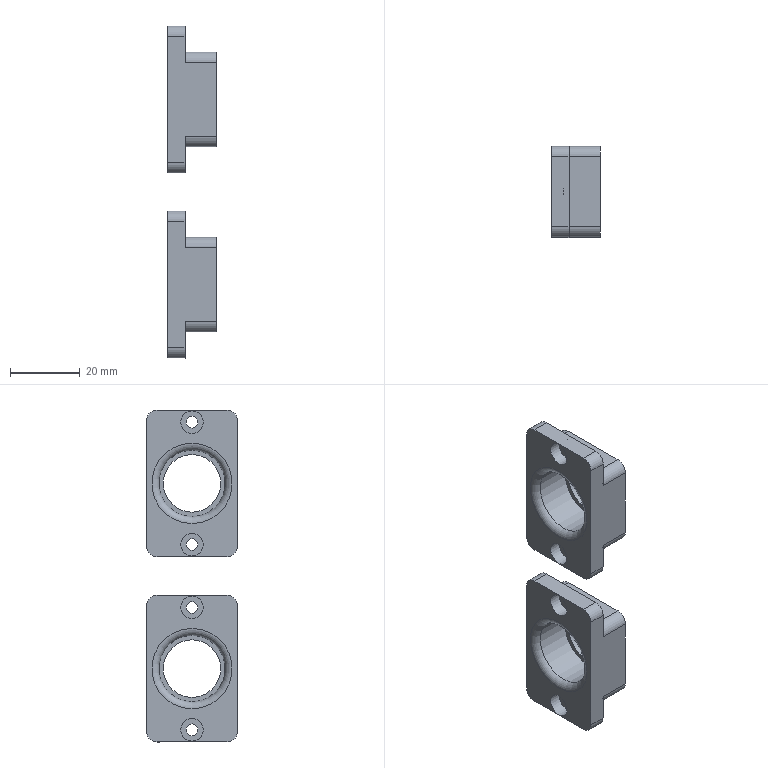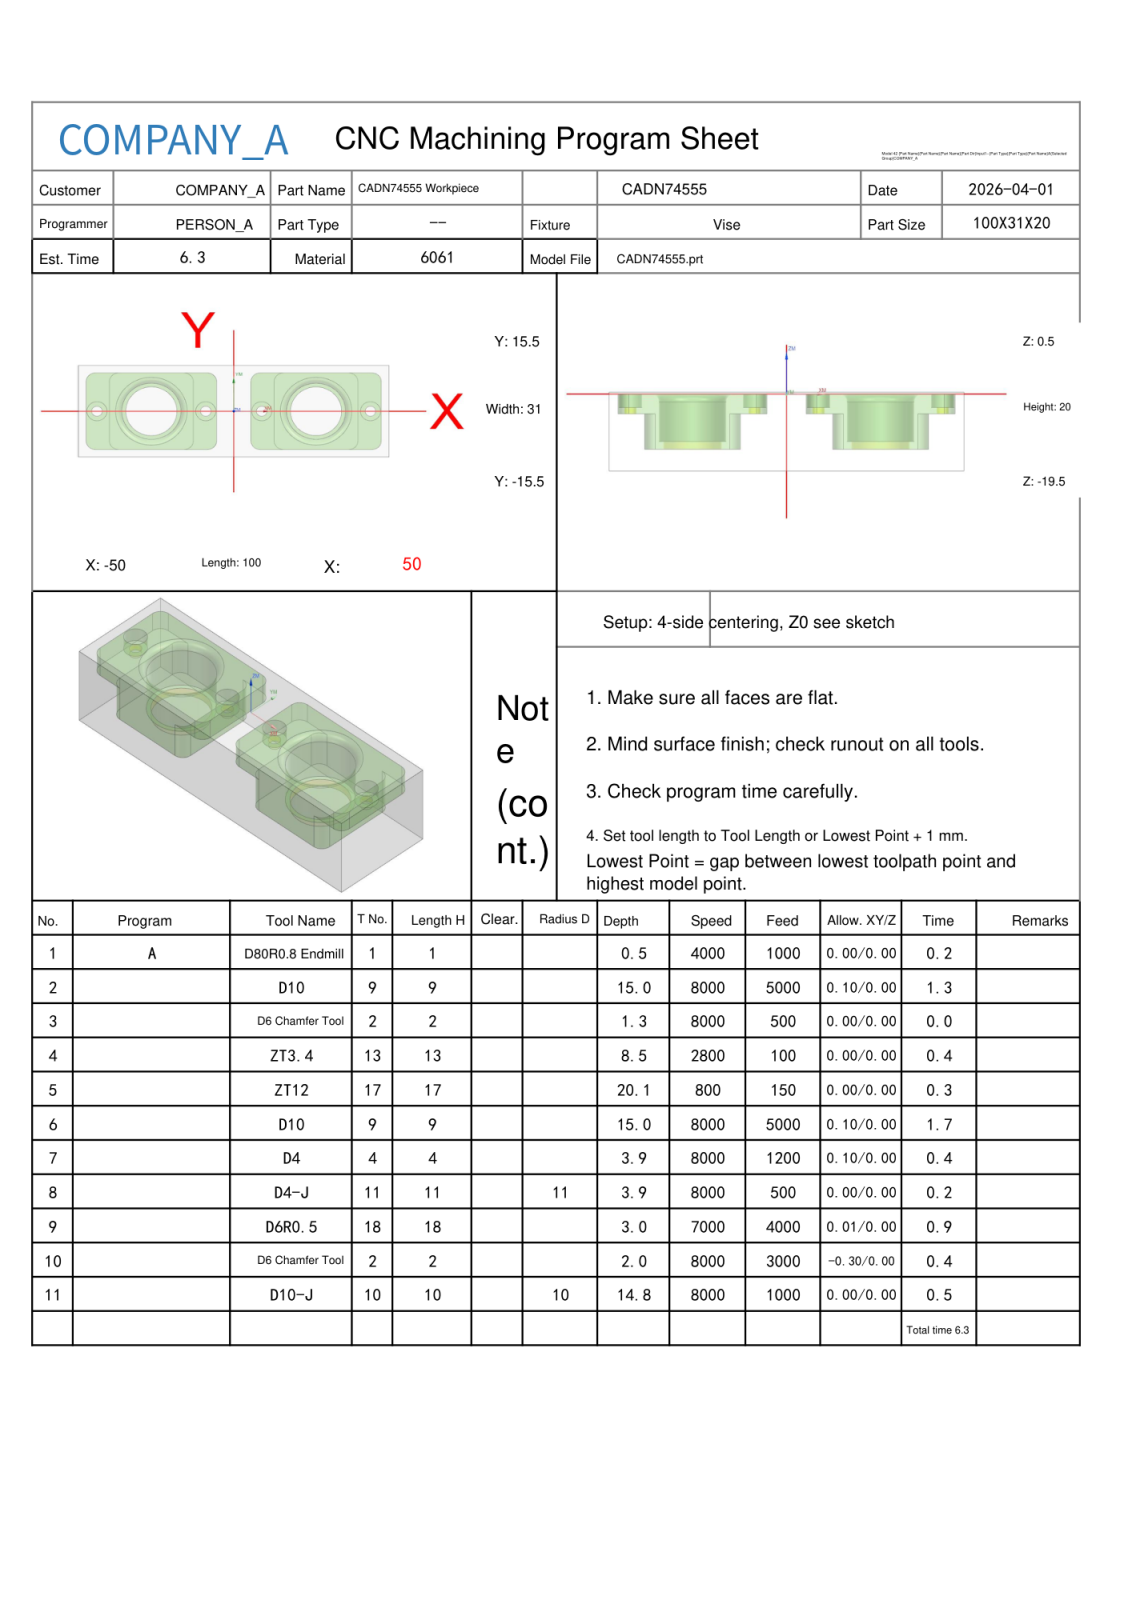NC program | NX | posted by the shop | part box 14 x 26 x 95 mm
Lines 5543 to 6944 of 19918:
N9 T18 M06
(D6R0.5  D=6. R=0.5 H=18 ce=0.01 di=0.00)
G00 G90 G54 X-25.418 Y8.734 M03 S7000
G43 H18 Z20.
M08
Z1.5
G01 X-25.945 Y8.792 Z1.472 F4000.
X-26.768 Y8.806 Z1.429
X-27.589 Y8.742 Z1.386
X-28.401 Y8.602 Z1.343
X-29.195 Y8.387 Z1.3
X-29.967 Y8.099 Z1.256
X-30.708 Y7.74 Z1.213
X-31.412 Y7.313 Z1.17
X-32.073 Y6.823 Z1.127
X-32.686 Y6.273 Z1.084
X-33.245 Y5.668 Z1.041
X-33.744 Y5.013 Z.998
X-34.066 Y4.514 Z.966
X-34.46 Y3.775 Z.923
X-34.782 Y3.003 Z.879
X-35.03 Y2.203 Z.835
X-35.201 Y1.384 Z.791
X-35.293 Y.552 Z.747
X-35.305 Y-.285 Z.703
X-35.238 Y-1.12 Z.659
X-35.093 Y-1.944 Z.615
X-34.869 Y-2.751 Z.572
X-34.57 Y-3.533 Z.528
X-34.199 Y-4.283 Z.484
X-33.757 Y-4.994 Z.44
X-33.251 Y-5.661 Z.396
X-32.683 Y-6.276 Z.352
X-32.059 Y-6.834 Z.308
X-31.385 Y-7.331 Z.264
X-30.668 Y-7.762 Z.221
X-29.912 Y-8.122 Z.177
X-29.126 Y-8.41 Z.133
X-28.316 Y-8.621 Z.089
X-27.731 Y-8.723 Z.058
X-27.265 Y-8.777 Z.033
X-26.797 Y-8.805 Z.009
X-26.5 Z-.007
G03 X-17.695 Y0.0 I0.0 J8.805
X-26.5 Y8.805 I-8.805 J0.0
X-35.305 Y0.0 I0.0 J-8.805
X-26.5 Y-8.805 I8.805 J0.0
G01 X-26.286 Y-8.802
X-26.072 Y-8.794
X-25.853 Y-8.78
X-25.634 Y-8.761
X-25.347 Y-8.726
X-25.06 Y-8.683
X-24.77 Y-8.629
X-24.481 Y-8.566
X-24.196 Y-8.492
X-23.912 Y-8.41
X-23.632 Y-8.317
X-23.355 Y-8.216
X-23.082 Y-8.105 Z-.008
X-22.812 Y-7.985
X-22.547 Y-7.856
X-22.286 Y-7.719
X-22.03 Y-7.572
X-21.778 Y-7.418
X-21.533 Y-7.255
X-21.293 Y-7.083
X-21.175 Y-6.995
X-21.059 Y-6.904
X-20.944 Y-6.812
X-20.831 Y-6.717
X-20.719 Y-6.621
X-20.609 Y-6.523
X-20.501 Y-6.423
X-20.394 Y-6.321
X-20.289 Y-6.217
X-20.186 Y-6.112
X-20.085 Y-6.005
X-19.985 Y-5.896
X-19.887 Y-5.786
X-19.791 Y-5.674
X-19.698 Y-5.561
X-19.606 Y-5.446
X-19.515 Y-5.329
X-19.427 Y-5.211
X-19.341 Y-5.091
X-19.257 Y-4.97 Z-.009
X-19.175 Y-4.848
X-19.095 Y-4.724
X-19.017 Y-4.599
X-18.941 Y-4.473
X-18.796 Y-4.217
X-18.66 Y-3.956
X-18.532 Y-3.69
X-18.413 Y-3.421
X-18.304 Y-3.147
X-18.203 Y-2.871
X-18.113 Y-2.591
X-18.031 Y-2.308
X-17.959 Y-2.022
X-17.896 Y-1.735
X-17.844 Y-1.445
X-17.801 Y-1.154
X-17.768 Y-.861
X-17.744 Y-.568
X-17.731 Y-.274
X-17.727 Y.02 Z-.01
X-17.734 Y.314
X-17.75 Y.608
X-17.776 Y.901
X-17.811 Y1.193
X-17.857 Y1.484
X-17.912 Y1.773
X-17.977 Y2.06
X-18.051 Y2.344
X-18.136 Y2.626
X-18.229 Y2.905
X-18.332 Y3.18
X-18.443 Y3.452
X-18.565 Y3.72
X-18.694 Y3.984
X-18.833 Y4.243
X-18.98 Y4.498
X-18.997 Y4.526
X-19.014 Y4.554
X-19.15 Y4.769
X-19.291 Y4.98 Z-.011
X-19.459 Y5.212
X-19.634 Y5.44
X-19.816 Y5.661
X-20.005 Y5.877
X-20.202 Y6.086
X-20.405 Y6.289
X-20.615 Y6.484
X-20.831 Y6.673
X-21.053 Y6.855
X-21.28 Y7.029
X-21.514 Y7.196
X-21.752 Y7.355
X-21.996 Y7.506
X-22.245 Y7.649
X-22.498 Y7.784
X-22.755 Y7.91
X-23.016 Y8.028
X-23.282 Y8.137 Z-.012
X-23.55 Y8.238
X-23.821 Y8.329
X-24.096 Y8.412
X-24.373 Y8.486
X-24.652 Y8.55
X-24.933 Y8.606
X-25.216 Y8.652
X-25.5 Y8.689
X-25.785 Y8.716
X-26.071 Y8.734
X-26.357 Y8.743
X-26.644
X-26.93 Y8.733
X-27.216 Y8.713
X-27.501 Y8.685
X-27.784 Y8.647
X-28.067 Y8.599
X-28.348 Y8.543 Z-.013
X-28.626 Y8.477
X-28.903 Y8.403
X-29.176 Y8.319
X-29.447 Y8.227
X-29.715 Y8.125
X-29.979 Y8.015
X-30.239 Y7.896
X-30.496 Y7.769
X-30.748 Y7.633
X-30.995 Y7.49
X-31.238 Y7.338
X-31.475 Y7.179
X-31.707 Y7.011
X-31.934 Y6.837
X-32.154 Y6.654
X-32.369 Y6.466
X-32.577 Y6.269
X-32.779 Y6.067 Z-.014
X-32.974 Y5.857
X-33.162 Y5.642
X-33.343 Y5.42
X-33.516 Y5.193
X-33.662 Y4.989
X-33.802 Y4.781
X-33.821 Y4.751
X-33.84 Y4.722
X-33.991 Y4.478
X-34.133 Y4.23
X-34.267 Y3.977
X-34.393 Y3.72
X-34.51 Y3.459
X-34.619 Y3.194
X-34.719 Y2.926
X-34.81 Y2.654
X-34.892 Y2.38
X-34.965 Y2.103
X-35.029 Y1.825
X-35.084 Y1.544
X-35.129 Y1.261 Z-.015
X-35.166 Y.977
X-35.192 Y.693
X-35.21 Y.407
X-35.218 Y.121
X-35.217 Y-.165
X-35.206 Y-.451
X-35.186 Y-.736
X-35.157 Y-1.021
X-35.118 Y-1.304
X-35.07 Y-1.586
X-35.013 Y-1.866
X-34.947 Y-2.144
X-34.872 Y-2.42
X-34.787 Y-2.693
X-34.694 Y-2.963
X-34.592 Y-3.23
X-34.481 Y-3.494
X-34.362 Y-3.754 Z-.016
X-34.234 Y-4.009
X-34.098 Y-4.261
X-33.954 Y-4.507
X-33.801 Y-4.749
X-33.641 Y-4.986
X-33.474 Y-5.217
X-33.298 Y-5.443
X-33.116 Y-5.662
X-32.926 Y-5.876
X-32.729 Y-6.083
X-32.526 Y-6.284
X-32.317 Y-6.478
X-32.101 Y-6.665
X-31.879 Y-6.845
X-31.651 Y-7.017
X-31.418 Y-7.182
X-31.179 Y-7.339
X-30.936 Y-7.488 Z-.017
X-30.688 Y-7.629
X-30.435 Y-7.762
X-30.178 Y-7.887
X-29.917 Y-8.002
X-29.653 Y-8.11
X-29.385 Y-8.208
X-29.114 Y-8.298
X-28.878 Y-8.368
X-28.642 Y-8.432
X-28.603 Y-8.441
X-28.564 Y-8.451
X-28.285 Y-8.513
X-28.005 Y-8.567
X-27.756 Y-8.606
X-27.506 Y-8.639
X-27.255 Y-8.664
X-27.004 Y-8.682
X-26.752 Y-8.692
X-26.5 Y-8.695
X-26.286 Y-8.692
X-26.072 Y-8.684 Z-.018
X-25.853 Y-8.67
X-25.635 Y-8.651
X-25.35 Y-8.617
X-25.066 Y-8.574
X-24.778 Y-8.52
X-24.493 Y-8.456
X-24.209 Y-8.383
X-23.929 Y-8.301
X-23.651 Y-8.209
X-23.377 Y-8.108
X-23.106 Y-7.998
X-22.839 Y-7.878
X-22.577 Y-7.75 Z-.019
X-22.319 Y-7.613
X-22.065 Y-7.468
X-21.817 Y-7.314
X-21.574 Y-7.152
X-21.336 Y-6.981
X-21.22 Y-6.893
X-21.105 Y-6.803
X-20.991 Y-6.711
X-20.879 Y-6.617
X-20.769 Y-6.522
X-20.66 Y-6.424
X-20.553 Y-6.325
X-20.448 Y-6.223
X-20.344 Y-6.12
X-20.242 Y-6.016
X-20.142 Y-5.91
X-20.044 Y-5.801
X-19.948 Y-5.692
X-19.853 Y-5.581
X-19.76 Y-5.468
X-19.67 Y-5.353 Z-.02
X-19.581 Y-5.238
X-19.494 Y-5.12
X-19.409 Y-5.002
X-19.326 Y-4.881
X-19.166 Y-4.637
X-19.015 Y-4.387
X-18.872 Y-4.133
X-18.738 Y-3.874
X-18.613 Y-3.61
X-18.496 Y-3.342
X-18.389 Y-3.071
X-18.291 Y-2.796
X-18.202 Y-2.518
X-18.122 Y-2.238
X-18.053 Y-1.954 Z-.021
X-17.992 Y-1.669
X-17.942 Y-1.382
X-17.9 Y-1.093
X-17.869 Y-.803
X-17.847 Y-.512
X-17.836 Y-.221
X-17.834 Y.071
X-17.842 Y.362
X-17.859 Y.653
X-17.887 Y.944
X-17.924 Y1.233
X-17.971 Y1.52
X-18.027 Y1.806 Z-.022
X-18.094 Y2.09
X-18.169 Y2.372
X-18.255 Y2.65
X-18.349 Y2.926
X-18.453 Y3.198
X-18.565 Y3.467
X-18.687 Y3.732
X-18.817 Y3.992
X-18.957 Y4.248
X-19.104 Y4.499
X-19.121 Y4.526
X-19.137 Y4.554
X-19.278 Y4.771
X-19.424 Y4.985
X-19.596 Y5.219 Z-.023
X-19.775 Y5.448
X-19.963 Y5.67
X-20.157 Y5.886
X-20.359 Y6.095
X-20.567 Y6.298
X-20.782 Y6.493
X-21.004 Y6.681
X-21.232 Y6.861
X-21.466 Y7.034
X-21.705 Y7.199
X-21.95 Y7.355
X-22.2 Y7.503 Z-.024
X-22.454 Y7.643
X-22.713 Y7.774
X-22.977 Y7.896
X-23.244 Y8.01
X-23.515 Y8.114
X-23.652 Y8.163
X-23.79 Y8.209
X-23.928 Y8.253
X-24.067 Y8.295
X-24.207 Y8.334
X-24.347 Y8.371
X-24.488 Y8.406
X-24.63 Y8.438
X-24.772 Y8.468
X-24.914 Y8.496
X-25.057 Y8.521
X-25.2 Y8.544
X-25.344 Y8.564
X-25.488 Y8.582
X-25.632 Y8.598
X-25.777 Y8.611 Z-.025
X-26.066 Y8.63
X-26.356 Y8.639
X-26.647 Y8.638
X-26.937 Y8.628
X-27.226 Y8.608
X-27.515 Y8.578
X-27.802 Y8.538
X-28.088 Y8.489
X-28.372 Y8.431
X-28.654 Y8.363
X-28.933 Y8.285
X-29.21 Y8.198
X-29.484 Y8.102 Z-.026
X-29.754 Y7.997
X-30.02 Y7.882
X-30.283 Y7.759
X-30.541 Y7.627
X-30.795 Y7.487
X-31.043 Y7.338
X-31.287 Y7.181
X-31.525 Y7.016
X-31.758 Y6.843
X-31.984 Y6.662
X-32.204 Y6.474
X-32.418 Y6.278
X-32.625 Y6.075 Z-.027
X-32.825 Y5.866
X-33.019 Y5.65
X-33.204 Y5.427
X-33.382 Y5.199
X-33.552 Y4.964
X-33.715 Y4.724
X-33.725 Y4.71
X-33.734 Y4.696
X-33.874 Y4.47
X-34.008 Y4.241
X-34.142 Y3.992
X-34.269 Y3.739
X-34.387 Y3.482
X-34.496 Y3.222
X-34.597 Y2.958 Z-.028
X-34.689 Y2.691
X-34.772 Y2.42
X-34.847 Y2.148
X-34.912 Y1.873
X-34.969 Y1.596
X-35.016 Y1.317
X-35.054 Y1.038
X-35.083 Y.756
X-35.103 Y.475
X-35.113 Y.192
X-35.114 Y-.09
X-35.106 Y-.372
X-35.089 Y-.654 Z-.029
X-35.062 Y-.936
X-35.027 Y-1.216
X-34.982 Y-1.494
X-34.928 Y-1.772
X-34.864 Y-2.047
X-34.792 Y-2.32
X-34.711 Y-2.59
X-34.622 Y-2.858
X-34.523 Y-3.122
X-34.416 Y-3.384
X-34.3 Y-3.641
X-34.176 Y-3.895
X-34.044 Y-4.144
X-33.904 Y-4.389 Z-.03
X-33.755 Y-4.629
X-33.599 Y-4.864
X-33.436 Y-5.094
X-33.264 Y-5.318
X-33.086 Y-5.537
X-32.901 Y-5.749
X-32.709 Y-5.956
X-32.51 Y-6.156
X-32.304 Y-6.349
X-32.093 Y-6.536
X-31.875 Y-6.715
X-31.652 Y-6.888
X-31.423 Y-7.052 Z-.031
X-31.189 Y-7.21
X-30.95 Y-7.359
X-30.706 Y-7.501
X-30.457 Y-7.634
X-30.205 Y-7.759
X-29.948 Y-7.876
X-29.688 Y-7.984
X-29.424 Y-8.084
X-29.158 Y-8.175
X-28.888 Y-8.257
X-28.616 Y-8.331
X-28.394 Y-8.384
X-28.17 Y-8.431 Z-.032
X-28.132 Y-8.438
X-28.094 Y-8.446
X-27.831 Y-8.49
X-27.566 Y-8.527
X-27.3 Y-8.556
X-27.034 Y-8.576
X-26.767 Y-8.588
X-26.5 Y-8.592
X-26.286 Y-8.589
X-26.072 Y-8.58
X-25.853 Y-8.566
X-25.635 Y-8.546
X-25.352 Y-8.512
X-25.071 Y-8.469
X-24.786 Y-8.415 Z-.033
X-24.503 Y-8.352
X-24.223 Y-8.279
X-23.945 Y-8.197
X-23.67 Y-8.106
X-23.398 Y-8.005
X-23.13 Y-7.895
X-22.866 Y-7.777
X-22.606 Y-7.649
X-22.35 Y-7.513
X-22.099 Y-7.368 Z-.034
X-21.853 Y-7.215
X-21.613 Y-7.053
X-21.378 Y-6.884
X-21.263 Y-6.796
X-21.149 Y-6.707
X-21.037 Y-6.615
X-20.926 Y-6.522
X-20.817 Y-6.426
X-20.71 Y-6.329
X-20.604 Y-6.231
X-20.5 Y-6.13
X-20.398 Y-6.028
X-20.297 Y-5.924
X-20.198 Y-5.818
X-20.101 Y-5.711
X-19.912 Y-5.491 Z-.035
X-19.731 Y-5.265
X-19.558 Y-5.034
X-19.393 Y-4.796
X-19.235 Y-4.553
X-19.086 Y-4.305
X-18.946 Y-4.052
X-18.814 Y-3.795
X-18.691 Y-3.533
X-18.576 Y-3.267
X-18.471 Y-2.998 Z-.036
X-18.375 Y-2.725
X-18.288 Y-2.449
X-18.211 Y-2.171
X-18.143 Y-1.889
X-18.085 Y-1.606
X-18.036 Y-1.321
X-17.996 Y-1.035
X-17.967 Y-.747
X-17.947 Y-.459
X-17.937 Y-.17 Z-.037
Y.119
X-17.947 Y.408
X-17.966 Y.696
X-17.995 Y.984
X-18.033 Y1.27
X-18.082 Y1.555
X-18.139 Y1.838
X-18.207 Y2.119
X-18.283 Y2.398
X-18.37 Y2.673 Z-.038
X-18.465 Y2.946
X-18.569 Y3.215
X-18.683 Y3.481
X-18.805 Y3.742
X-18.936 Y4.
X-19.076 Y4.252
X-19.224 Y4.5
X-19.241 Y4.527
X-19.258 Y4.554
X-19.398 Y4.767
X-19.543 Y4.977
X-19.714 Y5.207 Z-.039
X-19.893 Y5.431
X-20.079 Y5.649
X-20.273 Y5.861
X-20.473 Y6.066
X-20.68 Y6.264
X-20.894 Y6.455
X-21.114 Y6.639
X-21.34 Y6.815
X-21.572 Y6.984
X-21.809 Y7.145 Z-.04
X-22.051 Y7.298
X-22.299 Y7.442
X-22.551 Y7.579
X-22.807 Y7.706
X-23.068 Y7.825
X-23.332 Y7.935
X-23.601 Y8.037
X-23.872 Y8.129
X-24.146 Y8.212
X-24.423 Y8.286 Z-.041
X-24.702 Y8.35
X-24.983 Y8.405
X-25.266 Y8.451
X-25.55 Y8.487
X-25.835 Y8.513
X-26.12 Y8.53
X-26.407 Y8.538
X-26.693 Y8.536
X-26.979 Y8.524
X-27.264 Y8.502
X-27.549 Y8.471 Z-.042
X-27.832 Y8.431
X-28.114 Y8.381
X-28.394 Y8.322
X-28.672 Y8.253
X-28.947 Y8.175
X-29.22 Y8.088
X-29.489 Y7.992
X-29.755 Y7.887
X-30.018 Y7.772
X-30.276 Y7.65 Z-.043
X-30.53 Y7.518
X-30.78 Y7.379
X-31.024 Y7.23
X-31.264 Y7.074
X-31.498 Y6.91
X-31.727 Y6.738
X-31.949 Y6.559
X-32.166 Y6.372
X-32.376 Y6.178
X-32.579 Y5.978 Z-.044
X-32.776 Y5.77
X-32.965 Y5.556
X-33.147 Y5.336
X-33.322 Y5.11
X-33.489 Y4.878
X-33.649 Y4.64
X-33.691 Y4.573
X-33.734 Y4.506
X-33.84 Y4.329
X-33.943 Y4.149
X-34.078 Y3.896
X-34.205 Y3.639 Z-.045
X-34.322 Y3.377
X-34.431 Y3.112
X-34.53 Y2.843
X-34.621 Y2.572
X-34.702 Y2.297
X-34.775 Y2.02
X-34.837 Y1.74
X-34.891 Y1.459
X-34.934 Y1.175
X-34.969 Y.891 Z-.046
X-34.993 Y.606
X-35.008 Y.32
X-35.014 Y.033
X-35.01 Y-.253
X-34.996 Y-.539
X-34.972 Y-.824
X-34.939 Y-1.109
X-34.897 Y-1.392
X-34.845 Y-1.673
X-34.783 Y-1.953 Z-.047
X-34.712 Y-2.23
X-34.632 Y-2.505
X-34.543 Y-2.777
X-34.444 Y-3.046
X-34.337 Y-3.311
X-34.221 Y-3.572
X-34.096 Y-3.83
X-33.962 Y-4.083
X-33.82 Y-4.331
X-33.67 Y-4.575 Z-.048
X-33.512 Y-4.813
X-33.345 Y-5.046
X-33.171 Y-5.273
X-32.99 Y-5.494
X-32.801 Y-5.709
X-32.605 Y-5.917
X-32.402 Y-6.119
X-32.193 Y-6.313
X-31.977 Y-6.501
X-31.755 Y-6.681
X-31.527 Y-6.854 Z-.049
X-31.293 Y-7.019
X-31.054 Y-7.175
X-30.81 Y-7.324
X-30.561 Y-7.464
X-30.308 Y-7.596
X-30.05 Y-7.72
X-29.788 Y-7.834
X-29.523 Y-7.94
X-29.254 Y-8.037
X-28.982 Y-8.124 Z-.05
X-28.707 Y-8.203
X-28.43 Y-8.272
X-28.15 Y-8.332
X-27.878 Y-8.38
X-27.604 Y-8.42
X-27.566 Y-8.425
X-27.529 Y-8.43
X-27.291 Y-8.455
X-27.053 Y-8.474
X-26.777 Y-8.486
X-26.5 Y-8.49
X-26.286 Y-8.487 Z-.051
X-26.072 Y-8.479
X-25.858 Y-8.465
X-25.645 Y-8.446
X-25.516 Y-8.431
X-25.388 Y-8.415
X-25.232 Y-8.393
X-25.076 Y-8.367
X-24.794 Y-8.314
X-24.513 Y-8.251
X-24.235 Y-8.178
X-23.96 Y-8.096 Z-.052
X-23.688 Y-8.005
X-23.419 Y-7.905
X-23.153 Y-7.795
X-22.891 Y-7.677
X-22.634 Y-7.55
X-22.381 Y-7.414
X-22.133 Y-7.27
X-21.889 Y-7.118
X-21.651 Y-6.957 Z-.053
X-21.419 Y-6.788
X-21.192 Y-6.612
X-20.972 Y-6.428
X-20.758 Y-6.237
X-20.551 Y-6.039
X-20.35 Y-5.833
X-20.157 Y-5.622
X-19.97 Y-5.403 Z-.054
X-19.792 Y-5.179
X-19.621 Y-4.948
X-19.458 Y-4.712
X-19.303 Y-4.471
X-19.156 Y-4.225
X-19.018 Y-3.973
X-18.888 Y-3.718
X-18.767 Y-3.458 Z-.055
X-18.655 Y-3.194
X-18.552 Y-2.926
X-18.458 Y-2.655
X-18.373 Y-2.381
X-18.298 Y-2.105
X-18.232 Y-1.826
X-18.175 Y-1.545
X-18.128 Y-1.262 Z-.056
X-18.091 Y-.978
X-18.063 Y-.693
X-18.045 Y-.407
X-18.037 Y-.12
X-18.038 Y.166
X-18.049 Y.452
X-18.07 Y.738
X-18.1 Y1.023 Z-.057
X-18.14 Y1.307
X-18.19 Y1.589
X-18.249 Y1.869
X-18.318 Y2.147
X-18.395 Y2.423
X-18.483 Y2.695
X-18.579 Y2.965
X-18.684 Y3.231
X-18.799 Y3.494 Z-.058
X-18.922 Y3.752
X-19.054 Y4.006
X-19.194 Y4.256
X-19.343 Y4.5
X-19.36 Y4.527
X-19.377 Y4.554
X-19.517 Y4.765
X-19.663 Y4.972
X-19.835 Y5.199
X-20.014 Y5.42 Z-.059
X-20.201 Y5.635
X-20.395 Y5.844
X-20.596 Y6.046
X-20.804 Y6.242
X-21.018 Y6.43
X-21.238 Y6.61
X-21.464 Y6.784
X-21.696 Y6.949 Z-.06
X-21.933 Y7.107
X-22.176 Y7.256
X-22.423 Y7.397
X-22.675 Y7.53
X-22.931 Y7.654
X-23.192 Y7.77
X-23.456 Y7.876
X-23.723 Y7.974
X-23.994 Y8.062 Z-.061
X-24.267 Y8.142
X-24.543 Y8.212
X-24.821 Y8.273
X-25.101 Y8.324
X-25.382 Y8.366
X-25.665 Y8.398
X-25.949 Y8.421
X-26.233 Y8.435 Z-.062
X-26.518 Y8.438
X-26.802 Y8.432
X-27.086 Y8.417
X-27.369 Y8.392
X-27.652 Y8.357
X-27.933 Y8.313
X-28.212 Y8.259
X-28.489 Y8.197 Z-.063
X-28.765 Y8.124
X-29.037 Y8.043
X-29.306 Y7.952
X-29.573 Y7.853
X-29.836 Y7.744
X-30.094 Y7.627
X-30.349 Y7.501
X-30.6 Y7.366
X-30.846 Y7.223 Z-.064
X-31.086 Y7.072
X-31.322 Y6.913
X-31.552 Y6.746
X-31.776 Y6.572
X-31.994 Y6.39
X-32.206 Y6.201
X-32.412 Y6.004
X-32.61 Y5.801 Z-.065
X-32.802 Y5.592
X-32.987 Y5.376
X-33.164 Y5.154
X-33.333 Y4.926
X-33.468 Y4.733
X-33.597 Y4.537
X-33.623 Y4.495
X-33.649 Y4.454
X-33.793 Y4.212
X-33.93 Y3.965 Z-.066
X-34.057 Y3.714
X-34.177 Y3.46
X-34.288 Y3.201
X-34.39 Y2.938
X-34.483 Y2.673
X-34.568 Y2.404
X-34.643 Y2.133
X-34.71 Y1.859
X-34.767 Y1.584 Z-.067
X-34.815 Y1.306
X-34.853 Y1.028
X-34.882 Y.748
X-34.902 Y.467
X-34.912 Y.186
X-34.913 Y-.096
X-34.905 Y-.377
X-34.887 Y-.658 Z-.068
X-34.86 Y-.938
X-34.823 Y-1.216
X-34.778 Y-1.494
X-34.723 Y-1.77
X-34.658 Y-2.044
X-34.585 Y-2.315
X-34.503 Y-2.584
X-34.411 Y-2.85 Z-.069
X-34.311 Y-3.113
X-34.202 Y-3.372
X-34.085 Y-3.627
X-33.959 Y-3.879
X-33.824 Y-4.126
X-33.682 Y-4.368
X-33.531 Y-4.605
X-33.373 Y-4.838
X-33.207 Y-5.064 Z-.07
X-33.034 Y-5.286
X-32.853 Y-5.501
X-32.665 Y-5.71
X-32.47 Y-5.912
X-32.269 Y-6.108
X-32.061 Y-6.297
X-31.847 Y-6.479
X-31.627 Y-6.654 Z-.071
X-31.402 Y-6.821
X-31.171 Y-6.981
X-30.934 Y-7.133
X-30.693 Y-7.277
X-30.447 Y-7.413
X-30.197 Y-7.54
X-29.943 Y-7.659
X-29.684 Y-7.769
X-29.423 Y-7.871 Z-.072
X-29.158 Y-7.964
X-28.89 Y-8.048
X-28.619 Y-8.123
X-28.487 Y-8.156
X-28.354 Y-8.187
X-28.213 Y-8.217
X-28.072 Y-8.245
X-27.795 Y-8.293
X-27.517 Y-8.331
X-27.263 Y-8.357 Z-.073
X-27.009 Y-8.376
X-26.755 Y-8.387
X-26.5 Y-8.391
X-26.224 Y-8.386
X-25.949 Y-8.372
X-25.792 Y-8.36
X-25.635 Y-8.345
X-25.518 Y-8.331
X-25.401 Y-8.317
X-25.123 Y-8.274 Z-.074
X-24.847 Y-8.223
X-24.573 Y-8.163
X-24.301 Y-8.093
X-24.032 Y-8.014
X-23.765 Y-7.927
X-23.502 Y-7.83
X-23.242 Y-7.725 Z-.075
X-22.985 Y-7.611
X-22.733 Y-7.489
X-22.485 Y-7.358
X-22.241 Y-7.219
X-22.002 Y-7.072
X-21.768 Y-6.917
X-21.54 Y-6.755 Z-.076
X-21.317 Y-6.584
X-21.1 Y-6.407
X-20.889 Y-6.222
X-20.684 Y-6.03
X-20.486 Y-5.832
X-20.294 Y-5.627
X-20.11 Y-5.416 Z-.077
X-19.933 Y-5.199
X-19.763 Y-4.976
X-19.601 Y-4.747
X-19.446 Y-4.513
X-19.3 Y-4.274
X-19.161 Y-4.031
X-19.031 Y-3.783
X-18.909 Y-3.53 Z-.078
X-18.796 Y-3.274
X-18.691 Y-3.014
X-18.595 Y-2.751
X-18.508 Y-2.485
X-18.43 Y-2.216
X-18.36 Y-1.945
X-18.3 Y-1.671 Z-.079
X-18.25 Y-1.396
X-18.208 Y-1.119
X-18.176 Y-.84
X-18.153 Y-.561
X-18.139 Y-.282
X-18.135 Y-.002
X-18.14 Y.278 Z-.08
X-18.155 Y.558
X-18.179 Y.837
X-18.212 Y1.114
X-18.254 Y1.391
X-18.306 Y1.666
X-18.367 Y1.939
X-18.437 Y2.21 Z-.081
X-18.516 Y2.479
X-18.604 Y2.744
X-18.7 Y3.007
X-18.806 Y3.266
X-18.92 Y3.521
X-19.043 Y3.773
X-19.174 Y4.02 Z-.082
X-19.255 Y4.164
X-19.34 Y4.308
X-19.399 Y4.404
X-19.46 Y4.5
X-19.614 Y4.733
X-19.777 Y4.96
X-19.947 Y5.181
X-20.124 Y5.397
X-20.308 Y5.606 Z-.083
X-20.499 Y5.81
X-20.697 Y6.006
X-20.901 Y6.196
X-21.111 Y6.379
X-21.327 Y6.556
X-21.55 Y6.724
X-21.777 Y6.885 Z-.084
X-22.01 Y7.039
X-22.248 Y7.184
X-22.49 Y7.322
X-22.737 Y7.451
X-22.989 Y7.572
X-23.244 Y7.685
X-23.502 Y7.789 Z-.085
X-23.764 Y7.884
X-24.029 Y7.97
X-24.297 Y8.048
X-24.567 Y8.116
X-24.839 Y8.176
X-25.113 Y8.226
X-25.389 Y8.267
X-25.666 Y8.3 Z-.086
X-25.943 Y8.322
X-26.221 Y8.336
X-26.5 Y8.34
X-26.778 Y8.335
X-27.057 Y8.32
X-27.334 Y8.296
X-27.611 Y8.263 Z-.087
X-27.886 Y8.221
X-28.16 Y8.17
X-28.431 Y8.109
X-28.701 Y8.04
X-28.968 Y7.961
X-29.232 Y7.874
X-29.494 Y7.778 Z-.088
X-29.752 Y7.673
X-30.006 Y7.56
X-30.256 Y7.438
X-30.502 Y7.308
X-30.744 Y7.17
X-30.98 Y7.024
X-31.212 Y6.87 Z-.089
X-31.439 Y6.708
X-31.66 Y6.539
X-31.875 Y6.363
X-32.084 Y6.179
X-32.287 Y5.989
X-32.483 Y5.792
X-32.673 Y5.589 Z-.09
X-32.856 Y5.379
X-33.031 Y5.164
X-33.2 Y4.942
X-33.347 Y4.735
X-33.489 Y4.523
X-33.501 Y4.503
X-33.514 Y4.484
X-33.663 Y4.241
X-33.803 Y3.993 Z-.091
X-33.935 Y3.74
X-34.059 Y3.483
X-34.173 Y3.223
X-34.278 Y2.958
X-34.374 Y2.69
X-34.461 Y2.419
X-34.539 Y2.145 Z-.092
X-34.607 Y1.868
X-34.666 Y1.589
X-34.715 Y1.309
X-34.754 Y1.027
X-34.784 Y.744
X-34.804 Y.46
X-34.815 Y.176 Z-.093
Y-.109
X-34.806 Y-.394
X-34.787 Y-.678
X-34.759 Y-.961
X-34.72 Y-1.243
X-34.673 Y-1.523
X-34.615 Y-1.802 Z-.094
X-34.548 Y-2.078
X-34.472 Y-2.352
X-34.386 Y-2.624
X-34.291 Y-2.892
X-34.187 Y-3.157
X-34.074 Y-3.418
X-33.952 Y-3.675 Z-.095
X-33.822 Y-3.927
X-33.683 Y-4.175
X-33.535 Y-4.418
X-33.379 Y-4.656
X-33.216 Y-4.889
X-33.044 Y-5.115
X-32.865 Y-5.336 Z-.096
X-32.678 Y-5.55
X-32.484 Y-5.758
X-32.283 Y-5.959
X-32.076 Y-6.153
X-31.861 Y-6.34
X-31.641 Y-6.52
X-31.415 Y-6.691 Z-.097
X-31.182 Y-6.855
X-30.945 Y-7.011
X-30.702 Y-7.159
X-30.454 Y-7.298
X-30.202 Y-7.428
X-29.945 Y-7.55
X-29.685 Y-7.663 Z-.098
X-29.421 Y-7.767
X-29.153 Y-7.862
X-28.882 Y-7.948
X-28.609 Y-8.024
X-28.333 Y-8.091
X-28.107 Y-8.139
X-27.879 Y-8.18
X-27.861 Y-8.183
X-27.843 Y-8.186
X-27.633 Y-8.217 Z-.099
X-27.422 Y-8.243
X-27.192 Y-8.265
X-26.962 Y-8.281
X-26.731 Y-8.29
X-26.5 Y-8.293
X-26.286 Y-8.29
X-26.072 Y-8.281
X-25.853 Y-8.266 Z-.1
X-25.635 Y-8.246
X-25.355 Y-8.211
X-25.077 Y-8.167
X-24.795 Y-8.112
X-24.515 Y-8.048
X-24.237 Y-7.974
X-23.963 Y-7.89 Z-.101
X-23.691 Y-7.797
X-23.423 Y-7.694
X-23.159 Y-7.583
X-22.898 Y-7.462
X-22.642 Y-7.332
X-22.391 Y-7.194 Z-.102
X-22.267 Y-7.121
X-22.145 Y-7.047
X-22.024 Y-6.97
X-21.904 Y-6.891
X-21.785 Y-6.81
X-21.668 Y-6.727
X-21.552 Y-6.642
X-21.438 Y-6.555
X-21.326 Y-6.467
X-21.215 Y-6.376
X-21.105 Y-6.283 Z-.103
X-20.997 Y-6.188
X-20.891 Y-6.092
X-20.787 Y-5.994
X-20.684 Y-5.894
X-20.583 Y-5.792
X-20.484 Y-5.688
X-20.386 Y-5.583
X-20.291 Y-5.476
X-20.197 Y-5.368
X-20.105 Y-5.258
X-20.015 Y-5.146
X-19.928 Y-5.033 Z-.104
X-19.842 Y-4.918
X-19.676 Y-4.684
X-19.518 Y-4.445
X-19.369 Y-4.2
X-19.228 Y-3.95
X-19.096 Y-3.696
X-18.973 Y-3.437 Z-.105
X-18.859 Y-3.174
X-18.754 Y-2.907
X-18.659 Y-2.637
X-18.573 Y-2.364
X-18.496 Y-2.087
X-18.429 Y-1.809 Z-.106
X-18.372 Y-1.528
X-18.324 Y-1.246
X-18.287 Y-.962
X-18.259 Y-.677
X-18.241 Y-.391
X-18.233 Y-.105 Z-.107
X-18.235 Y.182
X-18.247 Y.468
X-18.268 Y.753
X-18.3 Y1.038
X-18.341 Y1.321
X-18.392 Y1.603 Z-.108
X-18.453 Y1.883
X-18.524 Y2.16
X-18.604 Y2.435
X-18.694 Y2.707
X-18.793 Y2.975
X-18.901 Y3.24 Z-.109
X-19.018 Y3.501
X-19.144 Y3.758
X-19.279 Y4.01
X-19.423 Y4.258
X-19.438 Y4.282
X-19.453 Y4.308
X-19.587 Y4.518 Z-.11
X-19.727 Y4.725
X-19.891 Y4.95
X-20.062 Y5.17
X-20.241 Y5.384
X-20.426 Y5.592
X-20.619 Y5.793
X-20.818 Y5.988 Z-.111
X-21.024 Y6.176
X-21.236 Y6.357
X-21.454 Y6.531
X-21.678 Y6.697
X-21.907 Y6.855
X-22.141 Y7.006 Z-.112
X-22.38 Y7.149
X-22.624 Y7.283
X-22.872 Y7.41
X-23.125 Y7.527
X-23.381 Y7.636
X-23.641 Y7.737 Z-.113
X-23.904 Y7.829
X-24.169 Y7.911
X-24.438 Y7.985
X-24.709 Y8.049
X-24.982 Y8.105
X-25.256 Y8.151 Z-.114
X-25.532 Y8.188
X-25.809 Y8.215
X-26.087 Y8.233
X-26.365 Y8.242
X-26.643 Y8.241
X-26.921 Y8.231 Z-.115
X-27.199 Y8.212
X-27.475 Y8.183
X-27.751 Y8.145
X-28.025 Y8.098
X-28.297 Y8.041
X-28.568 Y7.975
X-28.836 Y7.901 Z-.116
X-29.101 Y7.817
X-29.363 Y7.724
X-29.622 Y7.623
X-29.877 Y7.512
X-30.129 Y7.394
X-30.376 Y7.266 Z-.117
X-30.619 Y7.131
X-30.857 Y6.987
X-31.09 Y6.836
X-31.318 Y6.677
X-31.54 Y6.51
X-31.757 Y6.336 Z-.118
X-31.967 Y6.154
X-32.171 Y5.966
X-32.369 Y5.771
X-32.56 Y5.569
X-32.744 Y5.361
X-32.921 Y5.147 Z-.119
X-33.091 Y4.927
X-33.23 Y4.734
X-33.364 Y4.537
X-33.386 Y4.504
X-33.408 Y4.47
X-33.556 Y4.231
X-33.696 Y3.988
X-33.827 Y3.739 Z-.12
X-33.951 Y3.486
X-34.065 Y3.229
X-34.17 Y2.969
X-34.267 Y2.705
X-34.354 Y2.438
X-34.432 Y2.168 Z-.121
X-34.502 Y1.895
X-34.561 Y1.62
X-34.611 Y1.344
X-34.652 Y1.066
X-34.683 Y.787
X-34.705 Y.506
X-34.717 Y.226 Z-.122
X-34.719 Y-.055
X-34.712 Y-.336
X-34.695 Y-.616
X-34.669 Y-.896
X-34.633 Y-1.175
X-34.587 Y-1.452 Z-.123
X-34.533 Y-1.727
X-34.468 Y-2.001
X-34.395 Y-2.272
X-34.312 Y-2.54
X-34.22 Y-2.805
X-34.119 Y-3.067 Z-.124
X-34.01 Y-3.326
X-33.891 Y-3.58
X-33.764 Y-3.831
X-33.628 Y-4.076
X-33.485 Y-4.317
X-33.333 Y-4.553 Z-.125
X-33.173 Y-4.784
X-33.005 Y-5.009
X-32.829 Y-5.228
X-32.647 Y-5.441
X-32.457 Y-5.647
X-32.26 Y-5.847 Z-.126
X-32.056 Y-6.04
X-31.846 Y-6.226
X-31.63 Y-6.405
X-31.408 Y-6.576
X-31.18 Y-6.74
X-30.947 Y-6.895 Z-.127
X-30.708 Y-7.043
X-30.465 Y-7.182
X-30.217 Y-7.313
X-29.965 Y-7.435
X-29.708 Y-7.549
X-29.448 Y-7.654 Z-.128
X-29.185 Y-7.749
X-28.918 Y-7.836
X-28.729 Y-7.892
X-28.538 Y-7.943
X-28.458 Y-7.963
X-28.377 Y-7.982
X-28.103 Y-8.041
X-27.827 Y-8.091 Z-.129
X-27.607 Y-8.123
X-27.387 Y-8.15
X-27.166 Y-8.171
X-26.944 Y-8.185
X-26.722 Y-8.194
X-26.5 Y-8.196
X-26.286 Y-8.193
X-26.072 Y-8.185 Z-.13
X-25.853 Y-8.17
X-25.635 Y-8.149
X-25.358 Y-8.114
X-25.082 Y-8.07
X-24.802 Y-8.015
X-24.525 Y-7.951 Z-.131
X-24.25 Y-7.877
X-23.978 Y-7.794
X-23.709 Y-7.701
X-23.444 Y-7.599
X-23.182 Y-7.487 Z-.132
X-22.924 Y-7.367
X-22.67 Y-7.238
X-22.422 Y-7.1
X-22.299 Y-7.028
X-22.178 Y-6.954
X-22.058 Y-6.877
X-21.939 Y-6.799
X-21.822 Y-6.718 Z-.133
X-21.706 Y-6.636
X-21.592 Y-6.551
X-21.479 Y-6.465
X-21.367 Y-6.377
X-21.258 Y-6.286
X-21.149 Y-6.194
X-21.043 Y-6.1
X-20.938 Y-6.004
X-20.835 Y-5.906
X-20.733 Y-5.807 Z-.134
X-20.633 Y-5.706
X-20.439 Y-5.498
X-20.252 Y-5.284
X-20.073 Y-5.063
X-19.901 Y-4.837
X-19.738 Y-4.604 Z-.135
X-19.582 Y-4.366
X-19.435 Y-4.123
X-19.297 Y-3.875
X-19.167 Y-3.622
X-19.046 Y-3.365 Z-.136
X-18.934 Y-3.104
X-18.832 Y-2.839
X-18.738 Y-2.571
X-18.654 Y-2.3
X-18.579 Y-2.026
X-18.514 Y-1.749 Z-.137
X-18.459 Y-1.471
X-18.413 Y-1.19
X-18.377 Y-.909
X-18.351 Y-.626
X-18.335 Y-.342 Z-.138
X-18.328 Y-.059
X-18.332 Y.225
X-18.345 Y.509
X-18.368 Y.792
X-18.401 Y1.074 Z-.139
X-18.444 Y1.354
X-18.496 Y1.633
X-18.559 Y1.91
X-18.63 Y2.184
X-18.711 Y2.456
X-18.802 Y2.725 Z-.14
X-18.902 Y2.991
X-19.011 Y3.253
X-19.129 Y3.511
X-19.255 Y3.764
X-19.391 Y4.013 Z-.141
X-19.535 Y4.258
X-19.551 Y4.282
X-19.566 Y4.307
X-19.704 Y4.52
X-19.847 Y4.729
X-20.016 Y4.956
X-20.192 Y5.177 Z-.142
X-20.375 Y5.392
X-20.566 Y5.601
X-20.764 Y5.802
X-20.968 Y5.997
X-21.18 Y6.185
X-21.397 Y6.365 Z-.143
X-21.621 Y6.537
X-21.851 Y6.702
X-22.086 Y6.859
X-22.326 Y7.007
X-22.572 Y7.147 Z-.144
X-22.822 Y7.278
X-23.076 Y7.4
X-23.335 Y7.514
X-23.597 Y7.619
X-23.863 Y7.714 Z-.145
X-24.132 Y7.8
X-24.404 Y7.877
X-24.678 Y7.945
X-24.954 Y8.002
X-25.232 Y8.051
X-25.512 Y8.089 Z-.146
X-25.792 Y8.118
X-26.074 Y8.137
X-26.356 Y8.146
X-26.638
X-26.92 Y8.136 Z-.147
X-27.202 Y8.116
X-27.482 Y8.086
X-27.762 Y8.047
X-28.039 Y7.998
X-28.315 Y7.939 Z-.148
X-28.589 Y7.871
X-28.86 Y7.793
X-29.129 Y7.707
X-29.394 Y7.61
X-29.655 Y7.505
X-29.913 Y7.391 Z-.149
X-30.167 Y7.268
X-30.416 Y7.136
X-30.66 Y6.996
X-30.9 Y6.847
X-31.134 Y6.69 Z-.15
X-31.363 Y6.525
X-31.585 Y6.353
X-31.802 Y6.172
X-32.012 Y5.985
X-32.216 Y5.79 Z-.151
X-32.412 Y5.588
X-32.602 Y5.38
X-32.784 Y5.165
X-32.959 Y4.944
X-33.126 Y4.717
X-33.285 Y4.484 Z-.152
X-33.347 Y4.388
X-33.408 Y4.291
X-33.492 Y4.153
X-33.573 Y4.012
X-33.705 Y3.769